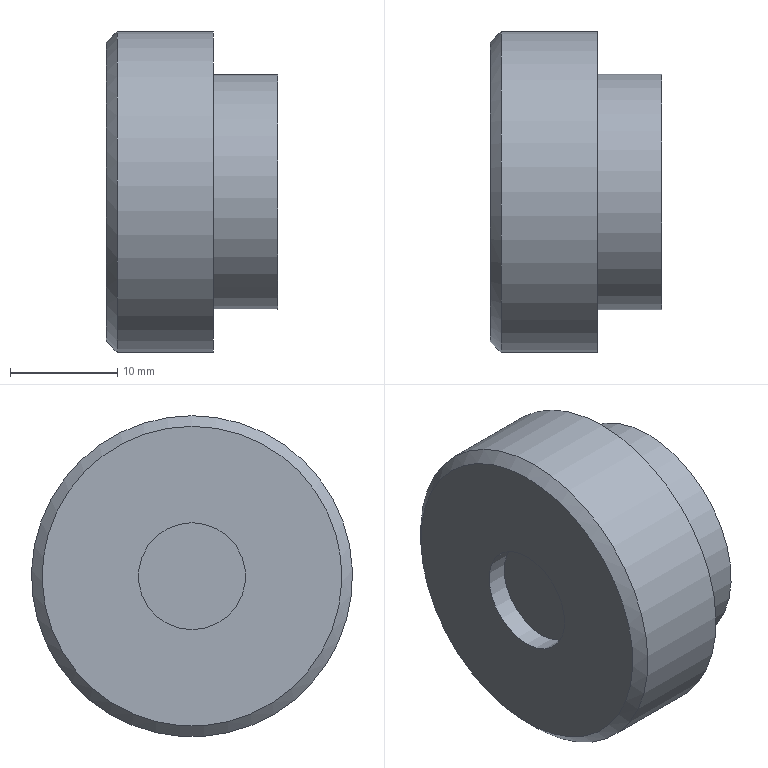Part | NX | features DATUM_CSYS 2, CHAMFER 1, SKETCH 1, SWP104 1, THREADS 1 | 1 solid | 15 faces | box 16 x 30 x 30 mm | volume 7540 mm3 | plane 6 | cylinder 6 | spline 2 | cone 1 | commonest cylinder face diameters 10 x1 10.3 x1 12 x1 16 x1 22 x1 30 x1
STEP:
#1=CARTESIAN_POINT('',(0.,0.,14.));
#2=VERTEX_POINT('',#1);
#3=CARTESIAN_POINT('',(0.,0.,0.));
#4=DIRECTION('',(-1.,0.,0.));
#5=DIRECTION('',(0.,0.,1.));
#6=AXIS2_PLACEMENT_3D('',#3,#4,#5);
#7=CIRCLE('',#6,14.);
#8=EDGE_CURVE('',#2,#2,#7,.T.);
#9=ORIENTED_EDGE('',*,*,#8,.T.);
#10=EDGE_LOOP('',(#9));
#11=FACE_BOUND('',#10,.T.);
#12=CARTESIAN_POINT('',(0.,0.,5.));
#13=VERTEX_POINT('',#12);
#14=CARTESIAN_POINT('',(0.,0.,0.));
#15=DIRECTION('',(-1.,0.,0.));
#16=DIRECTION('',(0.,0.,1.));
#17=AXIS2_PLACEMENT_3D('',#14,#15,#16);
#18=CIRCLE('',#17,5.);
#19=EDGE_CURVE('',#13,#13,#18,.T.);
#20=ORIENTED_EDGE('',*,*,#19,.F.);
#21=EDGE_LOOP('',(#20));
#22=FACE_BOUND('',#21,.T.);
#23=CARTESIAN_POINT('',(0.,5.,0.));
#24=DIRECTION('',(-1.,0.,0.));
#25=DIRECTION('',(0.,0.,1.));
#26=AXIS2_PLACEMENT_3D('',#23,#24,#25);
#27=PLANE('',#26);
#28=ADVANCED_FACE('',(#11,#22),#27,.T.);
#29=CARTESIAN_POINT('',(1.,0.,15.));
#30=VERTEX_POINT('',#29);
#31=CARTESIAN_POINT('',(1.,0.,0.));
#32=DIRECTION('',(-1.,0.,0.));
#33=DIRECTION('',(0.,0.,1.));
#34=AXIS2_PLACEMENT_3D('',#31,#32,#33);
#35=CIRCLE('',#34,15.);
#36=EDGE_CURVE('',#30,#30,#35,.F.);
#37=ORIENTED_EDGE('',*,*,#36,.T.);
#38=EDGE_LOOP('',(#37));
#39=FACE_BOUND('',#38,.T.);
#40=CARTESIAN_POINT('',(10.,0.,15.));
#41=VERTEX_POINT('',#40);
#42=CARTESIAN_POINT('',(10.,0.,0.));
#43=DIRECTION('',(-1.,0.,0.));
#44=DIRECTION('',(0.,0.,1.));
#45=AXIS2_PLACEMENT_3D('',#42,#43,#44);
#46=CIRCLE('',#45,15.);
#47=EDGE_CURVE('',#41,#41,#46,.T.);
#48=ORIENTED_EDGE('',*,*,#47,.T.);
#49=EDGE_LOOP('',(#48));
#50=FACE_BOUND('',#49,.T.);
#51=CARTESIAN_POINT('',(0.,0.,0.));
#52=DIRECTION('',(-1.,0.,0.));
#53=DIRECTION('',(0.,0.,1.));
#54=AXIS2_PLACEMENT_3D('',#51,#52,#53);
#55=CYLINDRICAL_SURFACE('',#54,15.);
#56=ADVANCED_FACE('',(#39,#50),#55,.T.);
#57=CARTESIAN_POINT('',(10.,0.,11.));
#58=VERTEX_POINT('',#57);
#59=CARTESIAN_POINT('',(10.,0.,0.));
#60=DIRECTION('',(-1.,0.,0.));
#61=DIRECTION('',(0.,0.,1.));
#62=AXIS2_PLACEMENT_3D('',#59,#60,#61);
#63=CIRCLE('',#62,11.);
#64=EDGE_CURVE('',#58,#58,#63,.T.);
#65=ORIENTED_EDGE('',*,*,#64,.T.);
#66=EDGE_LOOP('',(#65));
#67=FACE_BOUND('',#66,.T.);
#68=ORIENTED_EDGE('',*,*,#47,.F.);
#69=EDGE_LOOP('',(#68));
#70=FACE_BOUND('',#69,.T.);
#71=CARTESIAN_POINT('',(10.,15.,0.));
#72=DIRECTION('',(1.,0.,0.));
#73=DIRECTION('',(0.,0.,-1.));
#74=AXIS2_PLACEMENT_3D('',#71,#72,#73);
#75=PLANE('',#74);
#76=ADVANCED_FACE('',(#67,#70),#75,.T.);
#77=CARTESIAN_POINT('',(16.,0.,11.));
#78=VERTEX_POINT('',#77);
#79=CARTESIAN_POINT('',(16.,0.,0.));
#80=DIRECTION('',(-1.,0.,0.));
#81=DIRECTION('',(0.,0.,1.));
#82=AXIS2_PLACEMENT_3D('',#79,#80,#81);
#83=CIRCLE('',#82,11.);
#84=EDGE_CURVE('',#78,#78,#83,.T.);
#85=ORIENTED_EDGE('',*,*,#84,.T.);
#86=EDGE_LOOP('',(#85));
#87=FACE_BOUND('',#86,.T.);
#88=ORIENTED_EDGE('',*,*,#64,.F.);
#89=EDGE_LOOP('',(#88));
#90=FACE_BOUND('',#89,.T.);
#91=CARTESIAN_POINT('',(0.,0.,0.));
#92=DIRECTION('',(-1.,0.,0.));
#93=DIRECTION('',(0.,0.,1.));
#94=AXIS2_PLACEMENT_3D('',#91,#92,#93);
#95=CYLINDRICAL_SURFACE('',#94,11.);
#96=ADVANCED_FACE('',(#87,#90),#95,.T.);
#97=CARTESIAN_POINT('',(16.,4.694,-3.737));
#98=VERTEX_POINT('',#97);
#99=CARTESIAN_POINT('',(16.,2.383,4.566));
#100=VERTEX_POINT('',#99);
#101=CARTESIAN_POINT('',(16.,4.694,-3.737));
#102=CARTESIAN_POINT('',(16.,5.617,-2.363));
#103=CARTESIAN_POINT('',(16.,6.243,1.159));
#104=CARTESIAN_POINT('',(16.,3.919,3.938));
#105=CARTESIAN_POINT('',(16.,2.383,4.566));
#106=B_SPLINE_CURVE_WITH_KNOTS('',3,(#101,#102,#103,#104,#105),.UNSPECIFIED.,.F.,.F.,(4,1,4),(0.00006754,0.004972,0.009877),.UNSPECIFIED.);
#107=EDGE_CURVE('',#98,#100,#106,.T.);
#108=ORIENTED_EDGE('',*,*,#107,.F.);
#109=CARTESIAN_POINT('',(16.,-4.694,-3.737));
#110=VERTEX_POINT('',#109);
#111=CARTESIAN_POINT('',(16.,0.,0.));
#112=DIRECTION('',(1.,0.,0.));
#113=DIRECTION('',(0.,0.,-1.));
#114=AXIS2_PLACEMENT_3D('',#111,#112,#113);
#115=CIRCLE('',#114,6.);
#116=EDGE_CURVE('',#110,#98,#115,.T.);
#117=ORIENTED_EDGE('',*,*,#116,.F.);
#118=CARTESIAN_POINT('',(16.,-2.383,4.566));
#119=VERTEX_POINT('',#118);
#120=CARTESIAN_POINT('',(16.,-2.383,4.566));
#121=CARTESIAN_POINT('',(16.,-3.913,3.94));
#122=CARTESIAN_POINT('',(16.,-6.243,1.169));
#123=CARTESIAN_POINT('',(16.,-5.617,-2.363));
#124=CARTESIAN_POINT('',(16.,-4.694,-3.737));
#125=B_SPLINE_CURVE_WITH_KNOTS('',3,(#120,#121,#122,#123,#124),.UNSPECIFIED.,.F.,.F.,(4,1,4),(0.0001076,0.005014,0.00992),.UNSPECIFIED.);
#126=EDGE_CURVE('',#119,#110,#125,.T.);
#127=ORIENTED_EDGE('',*,*,#126,.F.);
#128=CARTESIAN_POINT('',(16.,0.,0.));
#129=DIRECTION('',(-1.,0.,0.));
#130=DIRECTION('',(0.,0.,1.));
#131=AXIS2_PLACEMENT_3D('',#128,#129,#130);
#132=CIRCLE('',#131,5.15);
#133=EDGE_CURVE('',#119,#100,#132,.T.);
#134=ORIENTED_EDGE('',*,*,#133,.T.);
#135=EDGE_LOOP('',(#108,#117,#127,#134));
#136=FACE_BOUND('',#135,.T.);
#137=ORIENTED_EDGE('',*,*,#84,.F.);
#138=EDGE_LOOP('',(#137));
#139=FACE_BOUND('',#138,.T.);
#140=CARTESIAN_POINT('',(16.,11.,0.));
#141=DIRECTION('',(1.,0.,0.));
#142=DIRECTION('',(0.,0.,-1.));
#143=AXIS2_PLACEMENT_3D('',#140,#141,#142);
#144=PLANE('',#143);
#145=ADVANCED_FACE('',(#136,#139),#144,.T.);
#146=CARTESIAN_POINT('',(12.,3.921,-3.339));
#147=VERTEX_POINT('',#146);
#148=CARTESIAN_POINT('',(16.,2.383,4.566));
#149=CARTESIAN_POINT('',(15.916,3.762,3.846));
#150=CARTESIAN_POINT('',(15.751,5.772,1.132));
#151=CARTESIAN_POINT('',(15.5,4.485,-3.821));
#152=CARTESIAN_POINT('',(15.25,-0.1879,-5.884));
#153=CARTESIAN_POINT('',(15.,-4.718,-3.525));
#154=CARTESIAN_POINT('',(14.75,-5.696,1.496));
#155=CARTESIAN_POINT('',(14.5,-2.387,5.382));
#156=CARTESIAN_POINT('',(14.25,2.721,5.224));
#157=CARTESIAN_POINT('',(14.,5.78,1.125));
#158=CARTESIAN_POINT('',(13.75,4.487,-3.812));
#159=CARTESIAN_POINT('',(13.5,-0.184,-5.887));
#160=CARTESIAN_POINT('',(13.25,-4.719,-3.523));
#161=CARTESIAN_POINT('',(13.001,-5.697,1.486));
#162=CARTESIAN_POINT('',(12.75,-2.39,5.384));
#163=CARTESIAN_POINT('',(12.5,2.723,5.223));
#164=CARTESIAN_POINT('',(12.25,5.773,1.13));
#165=CARTESIAN_POINT('',(12.085,4.93,-2.154));
#166=CARTESIAN_POINT('',(12.,3.921,-3.339));
#167=B_SPLINE_CURVE_WITH_KNOTS('',3,(#148,#149,#150,#151,#152,#153,#154,#155,#156,#157,#158,#159,#160,#161,#162,#163,#164,#165,#166),.UNSPECIFIED.,.F.,.F.,(4,1,1,1,1,1,1,1,1,1,1,1,1,1,1,1,4),(0.,0.004607,0.009214,0.01382,0.01843,0.02304,0.02764,0.03225,0.03686,0.04146,0.04607,0.05068,0.05528,0.05989,0.0645,0.06911,0.07371),.UNSPECIFIED.);
#168=EDGE_CURVE('',#100,#147,#167,.T.);
#169=ORIENTED_EDGE('',*,*,#168,.F.);
#170=ORIENTED_EDGE('',*,*,#133,.F.);
#171=CARTESIAN_POINT('',(12.,4.981,1.308));
#172=VERTEX_POINT('',#171);
#173=CARTESIAN_POINT('',(12.,4.981,1.308));
#174=CARTESIAN_POINT('',(12.084,4.586,2.813));
#175=CARTESIAN_POINT('',(12.25,2.387,5.376));
#176=CARTESIAN_POINT('',(12.5,-2.728,5.222));
#177=CARTESIAN_POINT('',(12.75,-5.779,1.125));
#178=CARTESIAN_POINT('',(13.,-4.486,-3.816));
#179=CARTESIAN_POINT('',(13.25,0.1916,-5.886));
#180=CARTESIAN_POINT('',(13.5,4.717,-3.524));
#181=CARTESIAN_POINT('',(13.75,5.698,1.491));
#182=CARTESIAN_POINT('',(14.,2.382,5.385));
#183=CARTESIAN_POINT('',(14.25,-2.719,5.222));
#184=CARTESIAN_POINT('',(14.5,-5.781,1.13));
#185=CARTESIAN_POINT('',(14.75,-4.484,-3.817));
#186=CARTESIAN_POINT('',(15.,0.1819,-5.885));
#187=CARTESIAN_POINT('',(15.25,4.717,-3.527));
#188=CARTESIAN_POINT('',(15.5,5.698,1.493));
#189=CARTESIAN_POINT('',(15.75,2.386,5.377));
#190=CARTESIAN_POINT('',(15.916,-1.004,5.285));
#191=CARTESIAN_POINT('',(16.,-2.383,4.566));
#192=B_SPLINE_CURVE_WITH_KNOTS('',3,(#173,#174,#175,#176,#177,#178,#179,#180,#181,#182,#183,#184,#185,#186,#187,#188,#189,#190,#191),.UNSPECIFIED.,.F.,.F.,(4,1,1,1,1,1,1,1,1,1,1,1,1,1,1,1,4),(0.,0.004607,0.009214,0.01382,0.01843,0.02303,0.02764,0.03225,0.03686,0.04146,0.04607,0.05068,0.05528,0.05989,0.0645,0.0691,0.07371),.UNSPECIFIED.);
#193=EDGE_CURVE('',#172,#119,#192,.T.);
#194=ORIENTED_EDGE('',*,*,#193,.F.);
#195=CARTESIAN_POINT('',(12.,0.,0.));
#196=DIRECTION('',(-1.,0.,0.));
#197=DIRECTION('',(0.,0.,1.));
#198=AXIS2_PLACEMENT_3D('',#195,#196,#197);
#199=CIRCLE('',#198,5.15);
#200=EDGE_CURVE('',#172,#147,#199,.T.);
#201=ORIENTED_EDGE('',*,*,#200,.T.);
#202=EDGE_LOOP('',(#169,#170,#194,#201));
#203=FACE_BOUND('',#202,.T.);
#204=CARTESIAN_POINT('',(0.,0.,0.));
#205=DIRECTION('',(-1.,0.,0.));
#206=DIRECTION('',(0.,0.,1.));
#207=AXIS2_PLACEMENT_3D('',#204,#205,#206);
#208=CYLINDRICAL_SURFACE('',#207,5.15);
#209=ADVANCED_FACE('',(#203),#208,.F.);
#210=CARTESIAN_POINT('',(12.,-2.597,5.409));
#211=VERTEX_POINT('',#210);
#212=CARTESIAN_POINT('',(12.,-2.597,5.409));
#213=CARTESIAN_POINT('',(12.,-1.053,6.004));
#214=CARTESIAN_POINT('',(12.,2.518,5.828));
#215=CARTESIAN_POINT('',(12.,4.712,2.946));
#216=CARTESIAN_POINT('',(12.,4.981,1.308));
#217=B_SPLINE_CURVE_WITH_KNOTS('',3,(#212,#213,#214,#215,#216),.UNSPECIFIED.,.F.,.F.,(4,1,4),(0.00006943,0.004974,0.009878),.UNSPECIFIED.);
#218=EDGE_CURVE('',#211,#172,#217,.T.);
#219=ORIENTED_EDGE('',*,*,#218,.F.);
#220=CARTESIAN_POINT('',(12.,-4.688,-3.745));
#221=VERTEX_POINT('',#220);
#222=CARTESIAN_POINT('',(12.,0.,0.));
#223=DIRECTION('',(-1.,0.,0.));
#224=DIRECTION('',(0.,0.,1.));
#225=AXIS2_PLACEMENT_3D('',#222,#223,#224);
#226=CIRCLE('',#225,6.);
#227=EDGE_CURVE('',#221,#211,#226,.T.);
#228=ORIENTED_EDGE('',*,*,#227,.F.);
#229=CARTESIAN_POINT('',(12.,3.921,-3.339));
#230=CARTESIAN_POINT('',(12.,2.972,-4.692));
#231=CARTESIAN_POINT('',(12.,-0.2478,-6.347));
#232=CARTESIAN_POINT('',(12.,-3.555,-4.952));
#233=CARTESIAN_POINT('',(12.,-4.688,-3.745));
#234=B_SPLINE_CURVE_WITH_KNOTS('',3,(#229,#230,#231,#232,#233),.UNSPECIFIED.,.F.,.F.,(4,1,4),(0.0001073,0.005013,0.009918),.UNSPECIFIED.);
#235=EDGE_CURVE('',#147,#221,#234,.T.);
#236=ORIENTED_EDGE('',*,*,#235,.F.);
#237=ORIENTED_EDGE('',*,*,#200,.F.);
#238=EDGE_LOOP('',(#219,#228,#236,#237));
#239=FACE_BOUND('',#238,.T.);
#240=CARTESIAN_POINT('',(12.,0.,8.));
#241=VERTEX_POINT('',#240);
#242=CARTESIAN_POINT('',(12.,0.,0.));
#243=DIRECTION('',(-1.,0.,0.));
#244=DIRECTION('',(0.,0.,1.));
#245=AXIS2_PLACEMENT_3D('',#242,#243,#244);
#246=CIRCLE('',#245,8.);
#247=EDGE_CURVE('',#241,#241,#246,.T.);
#248=ORIENTED_EDGE('',*,*,#247,.T.);
#249=EDGE_LOOP('',(#248));
#250=FACE_BOUND('',#249,.T.);
#251=CARTESIAN_POINT('',(12.,5.15,0.));
#252=DIRECTION('',(-1.,0.,0.));
#253=DIRECTION('',(0.,0.,1.));
#254=AXIS2_PLACEMENT_3D('',#251,#252,#253);
#255=PLANE('',#254);
#256=ADVANCED_FACE('',(#239,#250),#255,.T.);
#257=CARTESIAN_POINT('',(6.,0.,8.));
#258=VERTEX_POINT('',#257);
#259=CARTESIAN_POINT('',(6.,0.,0.));
#260=DIRECTION('',(-1.,0.,0.));
#261=DIRECTION('',(0.,0.,1.));
#262=AXIS2_PLACEMENT_3D('',#259,#260,#261);
#263=CIRCLE('',#262,8.);
#264=EDGE_CURVE('',#258,#258,#263,.T.);
#265=ORIENTED_EDGE('',*,*,#264,.T.);
#266=EDGE_LOOP('',(#265));
#267=FACE_BOUND('',#266,.T.);
#268=ORIENTED_EDGE('',*,*,#247,.F.);
#269=EDGE_LOOP('',(#268));
#270=FACE_BOUND('',#269,.T.);
#271=CARTESIAN_POINT('',(0.,0.,0.));
#272=DIRECTION('',(-1.,0.,0.));
#273=DIRECTION('',(0.,0.,1.));
#274=AXIS2_PLACEMENT_3D('',#271,#272,#273);
#275=CYLINDRICAL_SURFACE('',#274,8.);
#276=ADVANCED_FACE('',(#267,#270),#275,.F.);
#277=ORIENTED_EDGE('',*,*,#264,.F.);
#278=EDGE_LOOP('',(#277));
#279=FACE_BOUND('',#278,.T.);
#280=CARTESIAN_POINT('',(6.,8.,0.));
#281=DIRECTION('',(1.,0.,0.));
#282=DIRECTION('',(0.,0.,-1.));
#283=AXIS2_PLACEMENT_3D('',#280,#281,#282);
#284=PLANE('',#283);
#285=ADVANCED_FACE('',(#279),#284,.T.);
#286=CARTESIAN_POINT('',(2.,0.,5.));
#287=VERTEX_POINT('',#286);
#288=CARTESIAN_POINT('',(2.,0.,0.));
#289=DIRECTION('',(-1.,0.,0.));
#290=DIRECTION('',(0.,0.,1.));
#291=AXIS2_PLACEMENT_3D('',#288,#289,#290);
#292=CIRCLE('',#291,5.);
#293=EDGE_CURVE('',#287,#287,#292,.T.);
#294=ORIENTED_EDGE('',*,*,#293,.T.);
#295=EDGE_LOOP('',(#294));
#296=FACE_BOUND('',#295,.T.);
#297=CARTESIAN_POINT('',(2.,0.,0.));
#298=DIRECTION('',(-1.,0.,0.));
#299=DIRECTION('',(0.,0.,1.));
#300=AXIS2_PLACEMENT_3D('',#297,#298,#299);
#301=PLANE('',#300);
#302=ADVANCED_FACE('',(#296),#301,.T.);
#303=ORIENTED_EDGE('',*,*,#19,.T.);
#304=EDGE_LOOP('',(#303));
#305=FACE_BOUND('',#304,.T.);
#306=ORIENTED_EDGE('',*,*,#293,.F.);
#307=EDGE_LOOP('',(#306));
#308=FACE_BOUND('',#307,.T.);
#309=CARTESIAN_POINT('',(0.,0.,0.));
#310=DIRECTION('',(-1.,0.,0.));
#311=DIRECTION('',(0.,0.,1.));
#312=AXIS2_PLACEMENT_3D('',#309,#310,#311);
#313=CYLINDRICAL_SURFACE('',#312,5.);
#314=ADVANCED_FACE('',(#305,#308),#313,.F.);
#315=ORIENTED_EDGE('',*,*,#116,.T.);
#316=CARTESIAN_POINT('',(16.,4.694,-3.737));
#317=CARTESIAN_POINT('',(15.916,3.58,-5.136));
#318=CARTESIAN_POINT('',(15.75,0.0006715,-6.861));
#319=CARTESIAN_POINT('',(15.5,-5.359,-4.282));
#320=CARTESIAN_POINT('',(15.25,-6.692,1.52));
#321=CARTESIAN_POINT('',(15.,-2.978,6.181));
#322=CARTESIAN_POINT('',(14.75,2.97,6.184));
#323=CARTESIAN_POINT('',(14.5,6.689,1.534));
#324=CARTESIAN_POINT('',(14.25,5.365,-4.276));
#325=CARTESIAN_POINT('',(14.,0.008736,-6.86));
#326=CARTESIAN_POINT('',(13.75,-5.361,-4.284));
#327=CARTESIAN_POINT('',(13.5,-6.689,1.524));
#328=CARTESIAN_POINT('',(13.25,-2.985,6.176));
#329=CARTESIAN_POINT('',(13.,2.971,6.186));
#330=CARTESIAN_POINT('',(12.75,6.687,1.53));
#331=CARTESIAN_POINT('',(12.5,5.371,-4.27));
#332=CARTESIAN_POINT('',(12.25,0.004907,-6.859));
#333=CARTESIAN_POINT('',(12.083,-3.566,-5.15));
#334=CARTESIAN_POINT('',(12.,-4.688,-3.745));
#335=B_SPLINE_CURVE_WITH_KNOTS('',3,(#316,#317,#318,#319,#320,#321,#322,#323,#324,#325,#326,#327,#328,#329,#330,#331,#332,#333,#334),.UNSPECIFIED.,.F.,.F.,(4,1,1,1,1,1,1,1,1,1,1,1,1,1,1,1,4),(0.01341,0.01878,0.02414,0.02951,0.03487,0.04024,0.04561,0.05097,0.05634,0.0617,0.06707,0.07243,0.0778,0.08316,0.08853,0.0939,0.09926),.UNSPECIFIED.);
#336=EDGE_CURVE('',#221,#98,#335,.F.);
#337=ORIENTED_EDGE('',*,*,#336,.F.);
#338=ORIENTED_EDGE('',*,*,#227,.T.);
#339=CARTESIAN_POINT('',(12.,-2.597,5.409));
#340=CARTESIAN_POINT('',(12.083,-4.211,4.634));
#341=CARTESIAN_POINT('',(12.25,-6.688,1.53));
#342=CARTESIAN_POINT('',(12.5,-5.367,-4.272));
#343=CARTESIAN_POINT('',(12.75,-0.009134,-6.862));
#344=CARTESIAN_POINT('',(13.,5.363,-4.28));
#345=CARTESIAN_POINT('',(13.25,6.689,1.519));
#346=CARTESIAN_POINT('',(13.5,2.986,6.179));
#347=CARTESIAN_POINT('',(13.75,-2.974,6.183));
#348=CARTESIAN_POINT('',(14.,-6.686,1.535));
#349=CARTESIAN_POINT('',(14.25,-5.371,-4.272));
#350=CARTESIAN_POINT('',(14.5,-0.003143,-6.861));
#351=CARTESIAN_POINT('',(14.75,5.357,-4.285));
#352=CARTESIAN_POINT('',(15.,6.692,1.519));
#353=CARTESIAN_POINT('',(15.25,2.98,6.18));
#354=CARTESIAN_POINT('',(15.5,-2.968,6.186));
#355=CARTESIAN_POINT('',(15.75,-6.686,1.533));
#356=CARTESIAN_POINT('',(15.916,-5.812,-2.332));
#357=CARTESIAN_POINT('',(16.,-4.694,-3.737));
#358=B_SPLINE_CURVE_WITH_KNOTS('',3,(#339,#340,#341,#342,#343,#344,#345,#346,#347,#348,#349,#350,#351,#352,#353,#354,#355,#356,#357),.UNSPECIFIED.,.F.,.F.,(4,1,1,1,1,1,1,1,1,1,1,1,1,1,1,1,4),(0.01752,0.02289,0.02825,0.03362,0.03898,0.04435,0.04972,0.05508,0.06045,0.06581,0.07118,0.07654,0.08191,0.08728,0.09264,0.09801,0.1034),.UNSPECIFIED.);
#359=EDGE_CURVE('',#110,#211,#358,.F.);
#360=ORIENTED_EDGE('',*,*,#359,.F.);
#361=EDGE_LOOP('',(#315,#337,#338,#360));
#362=FACE_BOUND('',#361,.T.);
#363=CARTESIAN_POINT('',(16.875,0.,0.));
#364=DIRECTION('',(-1.,0.,0.));
#365=DIRECTION('',(0.,0.,1.));
#366=AXIS2_PLACEMENT_3D('',#363,#364,#365);
#367=CYLINDRICAL_SURFACE('',#366,6.);
#368=ADVANCED_FACE('',(#362),#367,.F.);
#369=ORIENTED_EDGE('',*,*,#107,.T.);
#370=ORIENTED_EDGE('',*,*,#168,.T.);
#371=ORIENTED_EDGE('',*,*,#235,.T.);
#372=ORIENTED_EDGE('',*,*,#336,.T.);
#373=EDGE_LOOP('',(#369,#370,#371,#372));
#374=FACE_BOUND('',#373,.T.);
#375=CARTESIAN_POINT('',(16.024,1.929,4.769));
#376=CARTESIAN_POINT('',(16.023,1.942,4.764));
#377=CARTESIAN_POINT('',(15.986,2.579,4.504));
#378=CARTESIAN_POINT('',(15.912,3.733,3.733));
#379=CARTESIAN_POINT('',(15.803,4.877,2.02));
#380=CARTESIAN_POINT('',(15.693,5.279,0.));
#381=CARTESIAN_POINT('',(15.584,4.877,-2.02));
#382=CARTESIAN_POINT('',(15.475,3.733,-3.733));
#383=CARTESIAN_POINT('',(15.365,2.02,-4.877));
#384=CARTESIAN_POINT('',(15.256,0.,-5.279));
#385=CARTESIAN_POINT('',(15.146,-2.02,-4.877));
#386=CARTESIAN_POINT('',(15.037,-3.733,-3.733));
#387=CARTESIAN_POINT('',(14.928,-4.877,-2.02));
#388=CARTESIAN_POINT('',(14.818,-5.279,0.));
#389=CARTESIAN_POINT('',(14.709,-4.877,2.02));
#390=CARTESIAN_POINT('',(14.6,-3.733,3.733));
#391=CARTESIAN_POINT('',(14.49,-2.02,4.877));
#392=CARTESIAN_POINT('',(14.381,0.,5.279));
#393=CARTESIAN_POINT('',(14.271,2.02,4.877));
#394=CARTESIAN_POINT('',(14.162,3.733,3.733));
#395=CARTESIAN_POINT('',(14.053,4.877,2.02));
#396=CARTESIAN_POINT('',(13.943,5.279,0.));
#397=CARTESIAN_POINT('',(13.834,4.877,-2.02));
#398=CARTESIAN_POINT('',(13.725,3.733,-3.733));
#399=CARTESIAN_POINT('',(13.615,2.02,-4.877));
#400=CARTESIAN_POINT('',(13.506,0.,-5.279));
#401=CARTESIAN_POINT('',(13.396,-2.02,-4.877));
#402=CARTESIAN_POINT('',(13.287,-3.733,-3.733));
#403=CARTESIAN_POINT('',(13.178,-4.877,-2.02));
#404=CARTESIAN_POINT('',(13.068,-5.279,0.));
#405=CARTESIAN_POINT('',(12.959,-4.877,2.02));
#406=CARTESIAN_POINT('',(12.85,-3.733,3.733));
#407=CARTESIAN_POINT('',(12.74,-2.02,4.877));
#408=CARTESIAN_POINT('',(12.631,0.,5.279));
#409=CARTESIAN_POINT('',(12.521,2.02,4.877));
#410=CARTESIAN_POINT('',(12.412,3.733,3.733));
#411=CARTESIAN_POINT('',(12.303,4.877,2.02));
#412=CARTESIAN_POINT('',(12.193,5.279,0.));
#413=CARTESIAN_POINT('',(12.084,4.877,-2.02));
#414=CARTESIAN_POINT('',(11.975,3.733,-3.733));
#415=CARTESIAN_POINT('',(11.865,2.02,-4.877));
#416=CARTESIAN_POINT('',(11.756,0.,-5.279));
#417=CARTESIAN_POINT('',(11.646,-2.02,-4.877));
#418=CARTESIAN_POINT('',(11.554,-3.464,-3.912));
#419=CARTESIAN_POINT('',(11.498,-4.116,-3.107));
#420=CARTESIAN_POINT('',(11.479,-4.311,-2.807));
#421=CARTESIAN_POINT('',(16.521,2.251,5.568));
#422=CARTESIAN_POINT('',(16.52,2.267,5.561));
#423=CARTESIAN_POINT('',(16.483,3.01,5.257));
#424=CARTESIAN_POINT('',(16.409,4.357,4.357));
#425=CARTESIAN_POINT('',(16.3,5.693,2.358));
#426=CARTESIAN_POINT('',(16.19,6.162,0.));
#427=CARTESIAN_POINT('',(16.081,5.693,-2.358));
#428=CARTESIAN_POINT('',(15.972,4.357,-4.357));
#429=CARTESIAN_POINT('',(15.862,2.358,-5.693));
#430=CARTESIAN_POINT('',(15.753,0.,-6.162));
#431=CARTESIAN_POINT('',(15.644,-2.358,-5.693));
#432=CARTESIAN_POINT('',(15.534,-4.357,-4.357));
#433=CARTESIAN_POINT('',(15.425,-5.693,-2.358));
#434=CARTESIAN_POINT('',(15.315,-6.162,0.));
#435=CARTESIAN_POINT('',(15.206,-5.693,2.358));
#436=CARTESIAN_POINT('',(15.097,-4.357,4.357));
#437=CARTESIAN_POINT('',(14.987,-2.358,5.693));
#438=CARTESIAN_POINT('',(14.878,0.,6.162));
#439=CARTESIAN_POINT('',(14.769,2.358,5.693));
#440=CARTESIAN_POINT('',(14.659,4.357,4.357));
#441=CARTESIAN_POINT('',(14.55,5.693,2.358));
#442=CARTESIAN_POINT('',(14.44,6.162,0.));
#443=CARTESIAN_POINT('',(14.331,5.693,-2.358));
#444=CARTESIAN_POINT('',(14.222,4.357,-4.357));
#445=CARTESIAN_POINT('',(14.112,2.358,-5.693));
#446=CARTESIAN_POINT('',(14.003,0.,-6.162));
#447=CARTESIAN_POINT('',(13.894,-2.358,-5.693));
#448=CARTESIAN_POINT('',(13.784,-4.357,-4.357));
#449=CARTESIAN_POINT('',(13.675,-5.693,-2.358));
#450=CARTESIAN_POINT('',(13.565,-6.162,0.));
#451=CARTESIAN_POINT('',(13.456,-5.693,2.358));
#452=CARTESIAN_POINT('',(13.347,-4.357,4.357));
#453=CARTESIAN_POINT('',(13.237,-2.358,5.693));
#454=CARTESIAN_POINT('',(13.128,0.,6.162));
#455=CARTESIAN_POINT('',(13.019,2.358,5.693));
#456=CARTESIAN_POINT('',(12.909,4.357,4.357));
#457=CARTESIAN_POINT('',(12.8,5.693,2.358));
#458=CARTESIAN_POINT('',(12.69,6.162,0.));
#459=CARTESIAN_POINT('',(12.581,5.693,-2.358));
#460=CARTESIAN_POINT('',(12.472,4.357,-4.357));
#461=CARTESIAN_POINT('',(12.362,2.358,-5.693));
#462=CARTESIAN_POINT('',(12.253,0.,-6.162));
#463=CARTESIAN_POINT('',(12.144,-2.358,-5.693));
#464=CARTESIAN_POINT('',(12.051,-4.044,-4.567));
#465=CARTESIAN_POINT('',(11.996,-4.805,-3.626));
#466=CARTESIAN_POINT('',(11.976,-5.032,-3.277));
#467=B_SPLINE_SURFACE_WITH_KNOTS('',1,3,((#375,#376,#377,#378,#379,#380,#381,#382,#383,#384,#385,#386,#387,#388,#389,#390,#391,#392,#393,#394,#395,#396,#397,#398,#399,#400,#401,#402,#403,#404,#405,#406,#407,#408,#409,#410,#411,#412,#413,#414,#415,#416,#417,#418,#419,#420),(#421,#422,#423,#424,#425,#426,#427,#428,#429,#430,#431,#432,#433,#434,#435,#436,#437,#438,#439,#440,#441,#442,#443,#444,#445,#446,#447,#448,#449,#450,#451,#452,#453,#454,#455,#456,#457,#458,#459,#460,#461,#462,#463,#464,#465,#466)),.RULED_SURF.,.F.,.F.,.F.,(2,2),(4,1,1,1,1,1,1,1,1,1,1,1,1,1,1,1,1,1,1,1,1,1,1,1,1,1,1,1,1,1,1,1,1,1,1,1,1,1,1,1,1,1,1,4),(0.00406,0.7466),(0.01801,0.01841,0.03682,0.05523,0.07363,0.09204,0.1105,0.1289,0.1473,0.1657,0.1841,0.2025,0.2209,0.2393,0.2577,0.2761,0.2945,0.3129,0.3314,0.3498,0.3682,0.3866,0.405,0.4234,0.4418,0.4602,0.4786,0.497,0.5154,0.5338,0.5523,0.5707,0.5891,0.6075,0.6259,0.6443,0.6627,0.6811,0.6995,0.7179,0.7363,0.7547,0.7732,0.7829),.UNSPECIFIED.);
#468=ADVANCED_FACE('',(#374),#467,.F.);
#469=ORIENTED_EDGE('',*,*,#126,.T.);
#470=ORIENTED_EDGE('',*,*,#359,.T.);
#471=ORIENTED_EDGE('',*,*,#218,.T.);
#472=ORIENTED_EDGE('',*,*,#193,.T.);
#473=EDGE_LOOP('',(#469,#470,#471,#472));
#474=FACE_BOUND('',#473,.T.);
#475=CARTESIAN_POINT('',(16.024,-4.315,-4.177));
#476=CARTESIAN_POINT('',(15.989,-4.839,-3.636));
#477=CARTESIAN_POINT('',(15.917,-5.699,-2.326));
#478=CARTESIAN_POINT('',(15.81,-6.162,0.));
#479=CARTESIAN_POINT('',(15.7,-5.693,2.358));
#480=CARTESIAN_POINT('',(15.591,-4.357,4.357));
#481=CARTESIAN_POINT('',(15.481,-2.358,5.693));
#482=CARTESIAN_POINT('',(15.372,0.,6.162));
#483=CARTESIAN_POINT('',(15.263,2.358,5.693));
#484=CARTESIAN_POINT('',(15.153,4.357,4.357));
#485=CARTESIAN_POINT('',(15.044,5.693,2.358));
#486=CARTESIAN_POINT('',(14.935,6.162,0.));
#487=CARTESIAN_POINT('',(14.825,5.693,-2.358));
#488=CARTESIAN_POINT('',(14.716,4.357,-4.357));
#489=CARTESIAN_POINT('',(14.606,2.358,-5.693));
#490=CARTESIAN_POINT('',(14.497,0.,-6.162));
#491=CARTESIAN_POINT('',(14.388,-2.358,-5.693));
#492=CARTESIAN_POINT('',(14.278,-4.357,-4.357));
#493=CARTESIAN_POINT('',(14.169,-5.693,-2.358));
#494=CARTESIAN_POINT('',(14.06,-6.162,0.));
#495=CARTESIAN_POINT('',(13.95,-5.693,2.358));
#496=CARTESIAN_POINT('',(13.841,-4.357,4.357));
#497=CARTESIAN_POINT('',(13.731,-2.358,5.693));
#498=CARTESIAN_POINT('',(13.622,0.,6.162));
#499=CARTESIAN_POINT('',(13.513,2.358,5.693));
#500=CARTESIAN_POINT('',(13.403,4.357,4.357));
#501=CARTESIAN_POINT('',(13.294,5.693,2.358));
#502=CARTESIAN_POINT('',(13.185,6.162,0.));
#503=CARTESIAN_POINT('',(13.075,5.693,-2.358));
#504=CARTESIAN_POINT('',(12.966,4.357,-4.357));
#505=CARTESIAN_POINT('',(12.856,2.358,-5.693));
#506=CARTESIAN_POINT('',(12.747,0.,-6.162));
#507=CARTESIAN_POINT('',(12.638,-2.358,-5.693));
#508=CARTESIAN_POINT('',(12.528,-4.357,-4.357));
#509=CARTESIAN_POINT('',(12.419,-5.693,-2.358));
#510=CARTESIAN_POINT('',(12.31,-6.162,0.));
#511=CARTESIAN_POINT('',(12.2,-5.693,2.358));
#512=CARTESIAN_POINT('',(12.091,-4.357,4.357));
#513=CARTESIAN_POINT('',(11.981,-2.358,5.693));
#514=CARTESIAN_POINT('',(11.872,0.,6.162));
#515=CARTESIAN_POINT('',(11.763,2.358,5.693));
#516=CARTESIAN_POINT('',(11.653,4.357,4.357));
#517=CARTESIAN_POINT('',(11.559,5.511,2.63));
#518=CARTESIAN_POINT('',(11.501,5.854,1.417));
#519=CARTESIAN_POINT('',(11.479,5.929,0.9574));
#520=CARTESIAN_POINT('',(16.521,-3.697,-3.578));
#521=CARTESIAN_POINT('',(16.486,-4.145,-3.114));
#522=CARTESIAN_POINT('',(16.415,-4.882,-1.992));
#523=CARTESIAN_POINT('',(16.307,-5.279,0.));
#524=CARTESIAN_POINT('',(16.197,-4.877,2.02));
#525=CARTESIAN_POINT('',(16.088,-3.733,3.733));
#526=CARTESIAN_POINT('',(15.979,-2.02,4.877));
#527=CARTESIAN_POINT('',(15.869,0.,5.279));
#528=CARTESIAN_POINT('',(15.76,2.02,4.877));
#529=CARTESIAN_POINT('',(15.65,3.733,3.733));
#530=CARTESIAN_POINT('',(15.541,4.877,2.02));
#531=CARTESIAN_POINT('',(15.432,5.279,0.));
#532=CARTESIAN_POINT('',(15.322,4.877,-2.02));
#533=CARTESIAN_POINT('',(15.213,3.733,-3.733));
#534=CARTESIAN_POINT('',(15.104,2.02,-4.877));
#535=CARTESIAN_POINT('',(14.994,0.,-5.279));
#536=CARTESIAN_POINT('',(14.885,-2.02,-4.877));
#537=CARTESIAN_POINT('',(14.775,-3.733,-3.733));
#538=CARTESIAN_POINT('',(14.666,-4.877,-2.02));
#539=CARTESIAN_POINT('',(14.557,-5.279,0.));
#540=CARTESIAN_POINT('',(14.447,-4.877,2.02));
#541=CARTESIAN_POINT('',(14.338,-3.733,3.733));
#542=CARTESIAN_POINT('',(14.229,-2.02,4.877));
#543=CARTESIAN_POINT('',(14.119,0.,5.279));
#544=CARTESIAN_POINT('',(14.01,2.02,4.877));
#545=CARTESIAN_POINT('',(13.9,3.733,3.733));
#546=CARTESIAN_POINT('',(13.791,4.877,2.02));
#547=CARTESIAN_POINT('',(13.682,5.279,0.));
#548=CARTESIAN_POINT('',(13.572,4.877,-2.02));
#549=CARTESIAN_POINT('',(13.463,3.733,-3.733));
#550=CARTESIAN_POINT('',(13.354,2.02,-4.877));
#551=CARTESIAN_POINT('',(13.244,0.,-5.279));
#552=CARTESIAN_POINT('',(13.135,-2.02,-4.877));
#553=CARTESIAN_POINT('',(13.025,-3.733,-3.733));
#554=CARTESIAN_POINT('',(12.916,-4.877,-2.02));
#555=CARTESIAN_POINT('',(12.807,-5.279,0.));
#556=CARTESIAN_POINT('',(12.697,-4.877,2.02));
#557=CARTESIAN_POINT('',(12.588,-3.733,3.733));
#558=CARTESIAN_POINT('',(12.479,-2.02,4.877));
#559=CARTESIAN_POINT('',(12.369,0.,5.279));
#560=CARTESIAN_POINT('',(12.26,2.02,4.877));
#561=CARTESIAN_POINT('',(12.15,3.733,3.733));
#562=CARTESIAN_POINT('',(12.056,4.721,2.253));
#563=CARTESIAN_POINT('',(11.998,5.015,1.214));
#564=CARTESIAN_POINT('',(11.976,5.079,0.8201));
#565=B_SPLINE_SURFACE_WITH_KNOTS('',1,3,((#475,#476,#477,#478,#479,#480,#481,#482,#483,#484,#485,#486,#487,#488,#489,#490,#491,#492,#493,#494,#495,#496,#497,#498,#499,#500,#501,#502,#503,#504,#505,#506,#507,#508,#509,#510,#511,#512,#513,#514,#515,#516,#517,#518,#519),(#520,#521,#522,#523,#524,#525,#526,#527,#528,#529,#530,#531,#532,#533,#534,#535,#536,#537,#538,#539,#540,#541,#542,#543,#544,#545,#546,#547,#548,#549,#550,#551,#552,#553,#554,#555,#556,#557,#558,#559,#560,#561,#562,#563,#564)),.RULED_SURF.,.F.,.F.,.F.,(2,2),(4,1,1,1,1,1,1,1,1,1,1,1,1,1,1,1,1,1,1,1,1,1,1,1,1,1,1,1,1,1,1,1,1,1,1,1,1,1,1,1,1,1,4),(0.2534,0.9959),(0.1848,0.2025,0.2209,0.2393,0.2577,0.2761,0.2945,0.3129,0.3314,0.3498,0.3682,0.3866,0.405,0.4234,0.4418,0.4602,0.4786,0.497,0.5154,0.5338,0.5523,0.5707,0.5891,0.6075,0.6259,0.6443,0.6627,0.6811,0.6995,0.7179,0.7363,0.7547,0.7732,0.7916,0.81,0.8284,0.8468,0.8652,0.8836,0.902,0.9204,0.9388,0.9497),.UNSPECIFIED.);
#566=ADVANCED_FACE('',(#474),#565,.F.);
#567=ORIENTED_EDGE('',*,*,#36,.F.);
#568=EDGE_LOOP('',(#567));
#569=FACE_BOUND('',#568,.T.);
#570=ORIENTED_EDGE('',*,*,#8,.F.);
#571=EDGE_LOOP('',(#570));
#572=FACE_BOUND('',#571,.T.);
#573=CARTESIAN_POINT('',(0.,0.,0.));
#574=DIRECTION('',(1.,0.,0.));
#575=DIRECTION('',(0.,0.,-1.));
#576=AXIS2_PLACEMENT_3D('',#573,#574,#575);
#577=CONICAL_SURFACE('',#576,14.,0.7854);
#578=ADVANCED_FACE('',(#569,#572),#577,.T.);
#579=CLOSED_SHELL('',(#28,#56,#76,#96,#145,#209,#256,#276,#285,#302,#314,#368,#468,#566,#578));
#580=MANIFOLD_SOLID_BREP('',#579);
#581=(LENGTH_UNIT()NAMED_UNIT(*)SI_UNIT(.MILLI.,.METRE.));
#582=UNCERTAINTY_MEASURE_WITH_UNIT(LENGTH_MEASURE(0.0508),#581,'','');
#583=(NAMED_UNIT(*)PLANE_ANGLE_UNIT()SI_UNIT($,.RADIAN.));
#584=(NAMED_UNIT(*)SI_UNIT($,.STERADIAN.)SOLID_ANGLE_UNIT());
#585=(GEOMETRIC_REPRESENTATION_CONTEXT(3)GLOBAL_UNCERTAINTY_ASSIGNED_CONTEXT((#582))GLOBAL_UNIT_ASSIGNED_CONTEXT((#581,#583,#584))REPRESENTATION_CONTEXT('',''));
#586=ADVANCED_BREP_SHAPE_REPRESENTATION('',(#580),#585);